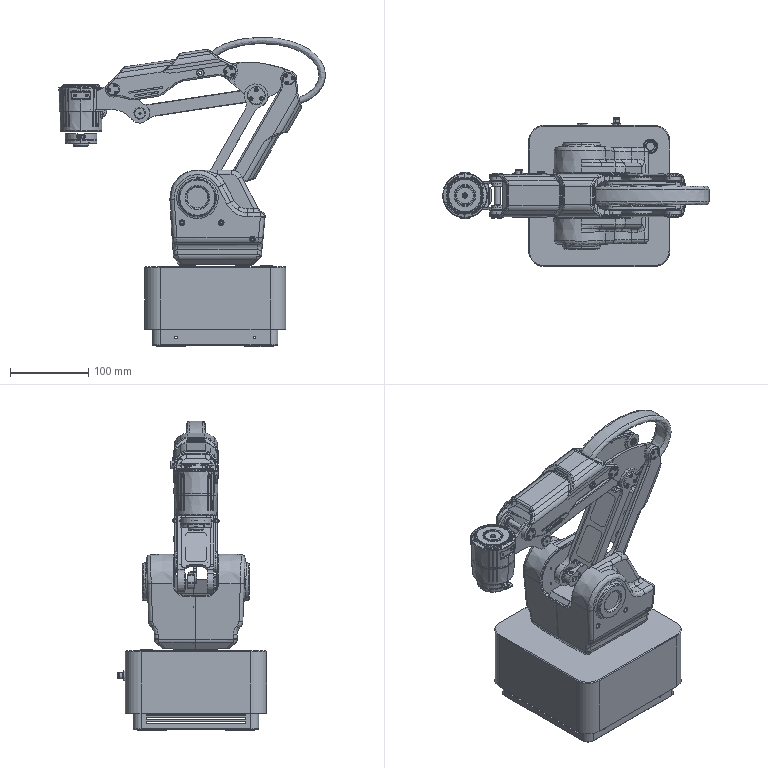Part | NX | features BREP 318, REPLACE_FACE 5, DATUM_CSYS 4, SKETCH 4, DELETE FACE 3, Delete Body 2, EXTRUDE 2, UNITE 1 | 362 solids | 11612 faces | volume 1159174 mm3 | plane 5142 | cylinder 3937 | spline 1246 | cone 720 | torus 386 | sphere 181 | commonest cylinder face diameters 1 x328 4 x300 2 x299 10 x191 2.5 x166 0.2 x163